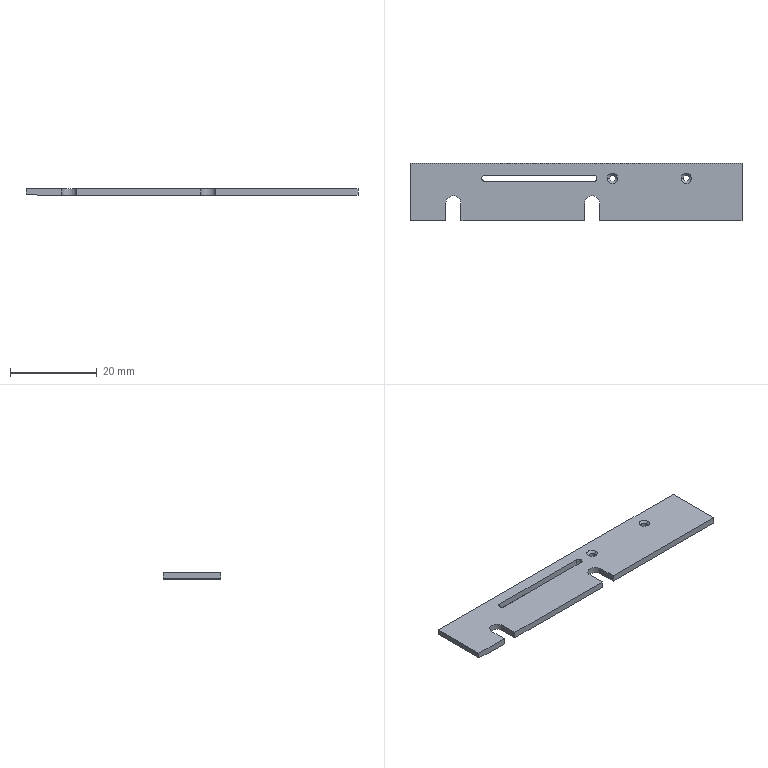Part | NX | 1 solid | 28 faces | box 76.5 x 13.2 x 1.5 mm | volume 1388 mm3 | plane 15 | cylinder 9 | cone 4 | commonest cylinder face diameters 1.4 x4 1.5 x3 3.5 x2
STEP:
#1=CARTESIAN_POINT('',(-191.15,-6.,0.75));
#2=VERTEX_POINT('',#1);
#3=CARTESIAN_POINT('',(-191.15,-2.,0.75));
#4=VERTEX_POINT('',#3);
#5=CARTESIAN_POINT('',(-191.15,0.,0.75));
#6=DIRECTION('',(0.,1.,0.));
#7=VECTOR('',#6,1000.);
#8=LINE('',#5,#7);
#9=EDGE_CURVE('',#2,#4,#8,.T.);
#10=ORIENTED_EDGE('',*,*,#9,.F.);
#11=CARTESIAN_POINT('',(-158.4,-6.,0.75));
#12=VERTEX_POINT('',#11);
#13=CARTESIAN_POINT('',(0.,-6.,0.75));
#14=DIRECTION('',(-1.,0.,0.));
#15=VECTOR('',#14,1000.);
#16=LINE('',#13,#15);
#17=EDGE_CURVE('',#12,#2,#16,.T.);
#18=ORIENTED_EDGE('',*,*,#17,.F.);
#19=CARTESIAN_POINT('',(-158.4,7.2,0.75));
#20=VERTEX_POINT('',#19);
#21=CARTESIAN_POINT('',(-158.4,0.,0.75));
#22=DIRECTION('',(0.,-1.,0.));
#23=VECTOR('',#22,1000.);
#24=LINE('',#21,#23);
#25=EDGE_CURVE('',#20,#12,#24,.T.);
#26=ORIENTED_EDGE('',*,*,#25,.F.);
#27=CARTESIAN_POINT('',(-234.9,7.2,0.75));
#28=VERTEX_POINT('',#27);
#29=CARTESIAN_POINT('',(0.,7.2,0.75));
#30=DIRECTION('',(1.,0.,0.));
#31=VECTOR('',#30,1000.);
#32=LINE('',#29,#31);
#33=EDGE_CURVE('',#28,#20,#32,.T.);
#34=ORIENTED_EDGE('',*,*,#33,.F.);
#35=CARTESIAN_POINT('',(-234.9,-6.,0.75));
#36=VERTEX_POINT('',#35);
#37=CARTESIAN_POINT('',(-234.9,0.,0.75));
#38=DIRECTION('',(0.,1.,0.));
#39=VECTOR('',#38,1000.);
#40=LINE('',#37,#39);
#41=EDGE_CURVE('',#36,#28,#40,.T.);
#42=ORIENTED_EDGE('',*,*,#41,.F.);
#43=CARTESIAN_POINT('',(-226.65,-6.,0.75));
#44=VERTEX_POINT('',#43);
#45=CARTESIAN_POINT('',(0.,-6.,0.75));
#46=DIRECTION('',(-1.,0.,0.));
#47=VECTOR('',#46,1000.);
#48=LINE('',#45,#47);
#49=EDGE_CURVE('',#44,#36,#48,.T.);
#50=ORIENTED_EDGE('',*,*,#49,.F.);
#51=CARTESIAN_POINT('',(-226.65,-2.,0.75));
#52=VERTEX_POINT('',#51);
#53=CARTESIAN_POINT('',(-226.65,0.,0.75));
#54=DIRECTION('',(0.,-1.,0.));
#55=VECTOR('',#54,1000.);
#56=LINE('',#53,#55);
#57=EDGE_CURVE('',#52,#44,#56,.T.);
#58=ORIENTED_EDGE('',*,*,#57,.F.);
#59=CARTESIAN_POINT('',(-223.15,-2.,0.75));
#60=VERTEX_POINT('',#59);
#61=CARTESIAN_POINT('',(-224.9,-2.,0.75));
#62=DIRECTION('',(0.,0.,-1.));
#63=DIRECTION('',(-1.,0.,0.));
#64=AXIS2_PLACEMENT_3D('',#61,#62,#63);
#65=CIRCLE('',#64,1.75);
#66=EDGE_CURVE('',#52,#60,#65,.T.);
#67=ORIENTED_EDGE('',*,*,#66,.T.);
#68=CARTESIAN_POINT('',(-223.15,-6.,0.75));
#69=VERTEX_POINT('',#68);
#70=CARTESIAN_POINT('',(-223.15,0.,0.75));
#71=DIRECTION('',(0.,1.,0.));
#72=VECTOR('',#71,1000.);
#73=LINE('',#70,#72);
#74=EDGE_CURVE('',#69,#60,#73,.T.);
#75=ORIENTED_EDGE('',*,*,#74,.F.);
#76=CARTESIAN_POINT('',(-194.65,-6.,0.75));
#77=VERTEX_POINT('',#76);
#78=CARTESIAN_POINT('',(0.,-6.,0.75));
#79=DIRECTION('',(-1.,0.,0.));
#80=VECTOR('',#79,1000.);
#81=LINE('',#78,#80);
#82=EDGE_CURVE('',#77,#69,#81,.T.);
#83=ORIENTED_EDGE('',*,*,#82,.F.);
#84=CARTESIAN_POINT('',(-194.65,-2.,0.75));
#85=VERTEX_POINT('',#84);
#86=CARTESIAN_POINT('',(-194.65,0.,0.75));
#87=DIRECTION('',(0.,-1.,0.));
#88=VECTOR('',#87,1000.);
#89=LINE('',#86,#88);
#90=EDGE_CURVE('',#85,#77,#89,.T.);
#91=ORIENTED_EDGE('',*,*,#90,.F.);
#92=CARTESIAN_POINT('',(-192.9,-2.,0.75));
#93=DIRECTION('',(0.,0.,-1.));
#94=DIRECTION('',(-1.,0.,0.));
#95=AXIS2_PLACEMENT_3D('',#92,#93,#94);
#96=CIRCLE('',#95,1.75);
#97=EDGE_CURVE('',#85,#4,#96,.T.);
#98=ORIENTED_EDGE('',*,*,#97,.T.);
#99=EDGE_LOOP('',(#10,#18,#26,#34,#42,#50,#58,#67,#75,#83,#91,#98));
#100=FACE_BOUND('',#99,.T.);
#101=CARTESIAN_POINT('',(-192.6,3.,0.75));
#102=VERTEX_POINT('',#101);
#103=CARTESIAN_POINT('',(-192.6,4.5,0.75));
#104=VERTEX_POINT('',#103);
#105=CARTESIAN_POINT('',(-192.6,3.75,0.75));
#106=DIRECTION('',(0.,0.,1.));
#107=DIRECTION('',(-1.,0.,0.));
#108=AXIS2_PLACEMENT_3D('',#105,#106,#107);
#109=CIRCLE('',#108,0.75);
#110=EDGE_CURVE('',#102,#104,#109,.T.);
#111=ORIENTED_EDGE('',*,*,#110,.F.);
#112=CARTESIAN_POINT('',(-217.6,3.,0.75));
#113=VERTEX_POINT('',#112);
#114=CARTESIAN_POINT('',(0.,3.,0.75));
#115=DIRECTION('',(1.,0.,0.));
#116=VECTOR('',#115,1000.);
#117=LINE('',#114,#116);
#118=EDGE_CURVE('',#113,#102,#117,.T.);
#119=ORIENTED_EDGE('',*,*,#118,.F.);
#120=CARTESIAN_POINT('',(-218.35,3.75,0.75));
#121=VERTEX_POINT('',#120);
#122=CARTESIAN_POINT('',(-217.6,3.75,0.75));
#123=DIRECTION('',(0.,0.,1.));
#124=DIRECTION('',(-1.,0.,0.));
#125=AXIS2_PLACEMENT_3D('',#122,#123,#124);
#126=CIRCLE('',#125,0.75);
#127=EDGE_CURVE('',#121,#113,#126,.T.);
#128=ORIENTED_EDGE('',*,*,#127,.F.);
#129=CARTESIAN_POINT('',(-217.6,4.5,0.75));
#130=VERTEX_POINT('',#129);
#131=CARTESIAN_POINT('',(-217.6,3.75,0.75));
#132=DIRECTION('',(0.,0.,1.));
#133=DIRECTION('',(-1.,0.,0.));
#134=AXIS2_PLACEMENT_3D('',#131,#132,#133);
#135=CIRCLE('',#134,0.75);
#136=EDGE_CURVE('',#130,#121,#135,.T.);
#137=ORIENTED_EDGE('',*,*,#136,.F.);
#138=CARTESIAN_POINT('',(0.,4.5,0.75));
#139=DIRECTION('',(-1.,0.,0.));
#140=VECTOR('',#139,1000.);
#141=LINE('',#138,#140);
#142=EDGE_CURVE('',#104,#130,#141,.T.);
#143=ORIENTED_EDGE('',*,*,#142,.F.);
#144=EDGE_LOOP('',(#111,#119,#128,#137,#143));
#145=FACE_BOUND('',#144,.T.);
#146=CARTESIAN_POINT('',(-189.45,3.75,0.75));
#147=VERTEX_POINT('',#146);
#148=CARTESIAN_POINT('',(-187.05,3.75,0.75));
#149=VERTEX_POINT('',#148);
#150=CARTESIAN_POINT('',(-188.25,3.75,0.75));
#151=DIRECTION('',(0.,0.,1.));
#152=DIRECTION('',(1.,0.,0.));
#153=AXIS2_PLACEMENT_3D('',#150,#151,#152);
#154=CIRCLE('',#153,1.2);
#155=EDGE_CURVE('',#147,#149,#154,.T.);
#156=ORIENTED_EDGE('',*,*,#155,.F.);
#157=CARTESIAN_POINT('',(-188.25,3.75,0.75));
#158=DIRECTION('',(0.,0.,1.));
#159=DIRECTION('',(1.,0.,0.));
#160=AXIS2_PLACEMENT_3D('',#157,#158,#159);
#161=CIRCLE('',#160,1.2);
#162=EDGE_CURVE('',#149,#147,#161,.T.);
#163=ORIENTED_EDGE('',*,*,#162,.F.);
#164=EDGE_LOOP('',(#156,#163));
#165=FACE_BOUND('',#164,.T.);
#166=CARTESIAN_POINT('',(-172.45,3.75,0.75));
#167=VERTEX_POINT('',#166);
#168=CARTESIAN_POINT('',(-170.05,3.75,0.75));
#169=VERTEX_POINT('',#168);
#170=CARTESIAN_POINT('',(-171.25,3.75,0.75));
#171=DIRECTION('',(0.,0.,1.));
#172=DIRECTION('',(1.,0.,0.));
#173=AXIS2_PLACEMENT_3D('',#170,#171,#172);
#174=CIRCLE('',#173,1.2);
#175=EDGE_CURVE('',#167,#169,#174,.T.);
#176=ORIENTED_EDGE('',*,*,#175,.F.);
#177=CARTESIAN_POINT('',(-171.25,3.75,0.75));
#178=DIRECTION('',(0.,0.,1.));
#179=DIRECTION('',(1.,0.,0.));
#180=AXIS2_PLACEMENT_3D('',#177,#178,#179);
#181=CIRCLE('',#180,1.2);
#182=EDGE_CURVE('',#169,#167,#181,.T.);
#183=ORIENTED_EDGE('',*,*,#182,.F.);
#184=EDGE_LOOP('',(#176,#183));
#185=FACE_BOUND('',#184,.T.);
#186=CARTESIAN_POINT('',(-196.6,0.,0.75));
#187=DIRECTION('',(0.,0.,-1.));
#188=DIRECTION('',(0.,-1.,0.));
#189=AXIS2_PLACEMENT_3D('',#186,#187,#188);
#190=PLANE('',#189);
#191=ADVANCED_FACE('',(#100,#145,#165,#185),#190,.F.);
#192=CARTESIAN_POINT('',(-191.15,-6.,-0.75));
#193=VERTEX_POINT('',#192);
#194=CARTESIAN_POINT('',(-191.15,-2.,-0.75));
#195=VERTEX_POINT('',#194);
#196=CARTESIAN_POINT('',(-191.15,0.,-0.75));
#197=DIRECTION('',(0.,1.,0.));
#198=VECTOR('',#197,1000.);
#199=LINE('',#196,#198);
#200=EDGE_CURVE('',#193,#195,#199,.T.);
#201=ORIENTED_EDGE('',*,*,#200,.F.);
#202=CARTESIAN_POINT('',(-191.15,-6.,0.));
#203=DIRECTION('',(0.,0.,1.));
#204=VECTOR('',#203,1000.);
#205=LINE('',#202,#204);
#206=EDGE_CURVE('',#193,#2,#205,.T.);
#207=ORIENTED_EDGE('',*,*,#206,.T.);
#208=ORIENTED_EDGE('',*,*,#9,.T.);
#209=CARTESIAN_POINT('',(-191.15,-2.,0.75));
#210=DIRECTION('',(0.,0.,-1.));
#211=VECTOR('',#210,1000.);
#212=LINE('',#209,#211);
#213=EDGE_CURVE('',#4,#195,#212,.T.);
#214=ORIENTED_EDGE('',*,*,#213,.T.);
#215=EDGE_LOOP('',(#201,#207,#208,#214));
#216=FACE_BOUND('',#215,.T.);
#217=CARTESIAN_POINT('',(-191.15,-6.,0.75));
#218=DIRECTION('',(1.,0.,0.));
#219=DIRECTION('',(0.,1.,0.));
#220=AXIS2_PLACEMENT_3D('',#217,#218,#219);
#221=PLANE('',#220);
#222=ADVANCED_FACE('',(#216),#221,.F.);
#223=ORIENTED_EDGE('',*,*,#213,.F.);
#224=ORIENTED_EDGE('',*,*,#97,.F.);
#225=CARTESIAN_POINT('',(-194.65,-2.,-0.75));
#226=VERTEX_POINT('',#225);
#227=CARTESIAN_POINT('',(-194.65,-2.,0.75));
#228=DIRECTION('',(0.,0.,-1.));
#229=VECTOR('',#228,1000.);
#230=LINE('',#227,#229);
#231=EDGE_CURVE('',#85,#226,#230,.T.);
#232=ORIENTED_EDGE('',*,*,#231,.T.);
#233=CARTESIAN_POINT('',(-192.9,-2.,-0.75));
#234=DIRECTION('',(0.,0.,-1.));
#235=DIRECTION('',(-1.,0.,0.));
#236=AXIS2_PLACEMENT_3D('',#233,#234,#235);
#237=CIRCLE('',#236,1.75);
#238=EDGE_CURVE('',#226,#195,#237,.T.);
#239=ORIENTED_EDGE('',*,*,#238,.T.);
#240=EDGE_LOOP('',(#223,#224,#232,#239));
#241=FACE_BOUND('',#240,.T.);
#242=CARTESIAN_POINT('',(-192.9,-2.,0.75));
#243=DIRECTION('',(0.,0.,-1.));
#244=DIRECTION('',(-1.,0.,0.));
#245=AXIS2_PLACEMENT_3D('',#242,#243,#244);
#246=CYLINDRICAL_SURFACE('',#245,1.75);
#247=ADVANCED_FACE('',(#241),#246,.F.);
#248=CARTESIAN_POINT('',(-194.65,-6.,-0.75));
#249=VERTEX_POINT('',#248);
#250=CARTESIAN_POINT('',(-194.65,0.,-0.75));
#251=DIRECTION('',(0.,-1.,0.));
#252=VECTOR('',#251,1000.);
#253=LINE('',#250,#252);
#254=EDGE_CURVE('',#226,#249,#253,.T.);
#255=ORIENTED_EDGE('',*,*,#254,.F.);
#256=ORIENTED_EDGE('',*,*,#231,.F.);
#257=ORIENTED_EDGE('',*,*,#90,.T.);
#258=CARTESIAN_POINT('',(-194.65,-6.,0.75));
#259=DIRECTION('',(0.,0.,-1.));
#260=VECTOR('',#259,1000.);
#261=LINE('',#258,#260);
#262=EDGE_CURVE('',#77,#249,#261,.T.);
#263=ORIENTED_EDGE('',*,*,#262,.T.);
#264=EDGE_LOOP('',(#255,#256,#257,#263));
#265=FACE_BOUND('',#264,.T.);
#266=CARTESIAN_POINT('',(-194.65,-2.,0.75));
#267=DIRECTION('',(-1.,0.,0.));
#268=DIRECTION('',(0.,0.,1.));
#269=AXIS2_PLACEMENT_3D('',#266,#267,#268);
#270=PLANE('',#269);
#271=ADVANCED_FACE('',(#265),#270,.F.);
#272=ORIENTED_EDGE('',*,*,#262,.F.);
#273=ORIENTED_EDGE('',*,*,#82,.T.);
#274=CARTESIAN_POINT('',(-223.15,-6.,-0.75));
#275=VERTEX_POINT('',#274);
#276=CARTESIAN_POINT('',(-223.15,-6.,0.75));
#277=DIRECTION('',(0.,0.,-1.));
#278=VECTOR('',#277,1000.);
#279=LINE('',#276,#278);
#280=EDGE_CURVE('',#69,#275,#279,.T.);
#281=ORIENTED_EDGE('',*,*,#280,.T.);
#282=CARTESIAN_POINT('',(0.,-6.,-0.75));
#283=DIRECTION('',(-1.,0.,0.));
#284=VECTOR('',#283,1000.);
#285=LINE('',#282,#284);
#286=EDGE_CURVE('',#249,#275,#285,.T.);
#287=ORIENTED_EDGE('',*,*,#286,.F.);
#288=EDGE_LOOP('',(#272,#273,#281,#287));
#289=FACE_BOUND('',#288,.T.);
#290=CARTESIAN_POINT('',(-158.3,-6.,-0.75));
#291=DIRECTION('',(0.,1.,0.));
#292=DIRECTION('',(1.,0.,0.));
#293=AXIS2_PLACEMENT_3D('',#290,#291,#292);
#294=PLANE('',#293);
#295=ADVANCED_FACE('',(#289),#294,.F.);
#296=CARTESIAN_POINT('',(-223.15,-2.,-0.75));
#297=VERTEX_POINT('',#296);
#298=CARTESIAN_POINT('',(-223.15,0.,-0.75));
#299=DIRECTION('',(0.,1.,0.));
#300=VECTOR('',#299,1000.);
#301=LINE('',#298,#300);
#302=EDGE_CURVE('',#275,#297,#301,.T.);
#303=ORIENTED_EDGE('',*,*,#302,.F.);
#304=ORIENTED_EDGE('',*,*,#280,.F.);
#305=ORIENTED_EDGE('',*,*,#74,.T.);
#306=CARTESIAN_POINT('',(-223.15,-2.,0.75));
#307=DIRECTION('',(0.,0.,-1.));
#308=VECTOR('',#307,1000.);
#309=LINE('',#306,#308);
#310=EDGE_CURVE('',#60,#297,#309,.T.);
#311=ORIENTED_EDGE('',*,*,#310,.T.);
#312=EDGE_LOOP('',(#303,#304,#305,#311));
#313=FACE_BOUND('',#312,.T.);
#314=CARTESIAN_POINT('',(-223.15,-6.,0.75));
#315=DIRECTION('',(1.,0.,0.));
#316=DIRECTION('',(0.,1.,0.));
#317=AXIS2_PLACEMENT_3D('',#314,#315,#316);
#318=PLANE('',#317);
#319=ADVANCED_FACE('',(#313),#318,.F.);
#320=ORIENTED_EDGE('',*,*,#310,.F.);
#321=ORIENTED_EDGE('',*,*,#66,.F.);
#322=CARTESIAN_POINT('',(-226.65,-2.,-0.75));
#323=VERTEX_POINT('',#322);
#324=CARTESIAN_POINT('',(-226.65,-2.,0.75));
#325=DIRECTION('',(0.,0.,-1.));
#326=VECTOR('',#325,1000.);
#327=LINE('',#324,#326);
#328=EDGE_CURVE('',#52,#323,#327,.T.);
#329=ORIENTED_EDGE('',*,*,#328,.T.);
#330=CARTESIAN_POINT('',(-224.9,-2.,-0.75));
#331=DIRECTION('',(0.,0.,-1.));
#332=DIRECTION('',(-1.,0.,0.));
#333=AXIS2_PLACEMENT_3D('',#330,#331,#332);
#334=CIRCLE('',#333,1.75);
#335=EDGE_CURVE('',#323,#297,#334,.T.);
#336=ORIENTED_EDGE('',*,*,#335,.T.);
#337=EDGE_LOOP('',(#320,#321,#329,#336));
#338=FACE_BOUND('',#337,.T.);
#339=CARTESIAN_POINT('',(-224.9,-2.,0.75));
#340=DIRECTION('',(0.,0.,-1.));
#341=DIRECTION('',(-1.,0.,0.));
#342=AXIS2_PLACEMENT_3D('',#339,#340,#341);
#343=CYLINDRICAL_SURFACE('',#342,1.75);
#344=ADVANCED_FACE('',(#338),#343,.F.);
#345=CARTESIAN_POINT('',(-226.65,-6.,-0.75));
#346=VERTEX_POINT('',#345);
#347=CARTESIAN_POINT('',(-226.65,0.,-0.75));
#348=DIRECTION('',(0.,-1.,0.));
#349=VECTOR('',#348,1000.);
#350=LINE('',#347,#349);
#351=EDGE_CURVE('',#323,#346,#350,.T.);
#352=ORIENTED_EDGE('',*,*,#351,.F.);
#353=ORIENTED_EDGE('',*,*,#328,.F.);
#354=ORIENTED_EDGE('',*,*,#57,.T.);
#355=CARTESIAN_POINT('',(-226.65,-6.,0.75));
#356=DIRECTION('',(0.,0.,-1.));
#357=VECTOR('',#356,1000.);
#358=LINE('',#355,#357);
#359=EDGE_CURVE('',#44,#346,#358,.T.);
#360=ORIENTED_EDGE('',*,*,#359,.T.);
#361=EDGE_LOOP('',(#352,#353,#354,#360));
#362=FACE_BOUND('',#361,.T.);
#363=CARTESIAN_POINT('',(-226.65,-2.,0.75));
#364=DIRECTION('',(-1.,0.,0.));
#365=DIRECTION('',(0.,0.,1.));
#366=AXIS2_PLACEMENT_3D('',#363,#364,#365);
#367=PLANE('',#366);
#368=ADVANCED_FACE('',(#362),#367,.F.);
#369=ORIENTED_EDGE('',*,*,#359,.F.);
#370=ORIENTED_EDGE('',*,*,#49,.T.);
#371=CARTESIAN_POINT('',(-234.9,-6.,-0.4875));
#372=VERTEX_POINT('',#371);
#373=CARTESIAN_POINT('',(-234.9,-6.,0.));
#374=DIRECTION('',(0.,0.,-1.));
#375=VECTOR('',#374,1000.);
#376=LINE('',#373,#375);
#377=EDGE_CURVE('',#36,#372,#376,.T.);
#378=ORIENTED_EDGE('',*,*,#377,.T.);
#379=CARTESIAN_POINT('',(-231.9,-6.,-0.75));
#380=VERTEX_POINT('',#379);
#381=CARTESIAN_POINT('',(0.,-6.,-21.039));
#382=DIRECTION('',(0.9962,0.,-0.08716));
#383=VECTOR('',#382,1000.);
#384=LINE('',#381,#383);
#385=EDGE_CURVE('',#372,#380,#384,.T.);
#386=ORIENTED_EDGE('',*,*,#385,.T.);
#387=CARTESIAN_POINT('',(0.,-6.,-0.75));
#388=DIRECTION('',(-1.,0.,0.));
#389=VECTOR('',#388,1000.);
#390=LINE('',#387,#389);
#391=EDGE_CURVE('',#346,#380,#390,.T.);
#392=ORIENTED_EDGE('',*,*,#391,.F.);
#393=EDGE_LOOP('',(#369,#370,#378,#386,#392));
#394=FACE_BOUND('',#393,.T.);
#395=CARTESIAN_POINT('',(-158.3,-6.,-0.75));
#396=DIRECTION('',(0.,1.,0.));
#397=DIRECTION('',(1.,0.,0.));
#398=AXIS2_PLACEMENT_3D('',#395,#396,#397);
#399=PLANE('',#398);
#400=ADVANCED_FACE('',(#394),#399,.F.);
#401=CARTESIAN_POINT('',(-231.9,7.2,-0.75));
#402=VERTEX_POINT('',#401);
#403=CARTESIAN_POINT('',(-231.9,0.,-0.75));
#404=DIRECTION('',(0.,1.,0.));
#405=VECTOR('',#404,1000.);
#406=LINE('',#403,#405);
#407=EDGE_CURVE('',#380,#402,#406,.T.);
#408=ORIENTED_EDGE('',*,*,#407,.F.);
#409=ORIENTED_EDGE('',*,*,#385,.F.);
#410=CARTESIAN_POINT('',(-234.9,7.2,-0.4875));
#411=VERTEX_POINT('',#410);
#412=CARTESIAN_POINT('',(-234.9,0.,-0.4875));
#413=DIRECTION('',(0.,1.,0.));
#414=VECTOR('',#413,1000.);
#415=LINE('',#412,#414);
#416=EDGE_CURVE('',#372,#411,#415,.T.);
#417=ORIENTED_EDGE('',*,*,#416,.T.);
#418=CARTESIAN_POINT('',(0.,7.2,-21.039));
#419=DIRECTION('',(0.9962,0.,-0.08716));
#420=VECTOR('',#419,1000.);
#421=LINE('',#418,#420);
#422=EDGE_CURVE('',#411,#402,#421,.T.);
#423=ORIENTED_EDGE('',*,*,#422,.T.);
#424=EDGE_LOOP('',(#408,#409,#417,#423));
#425=FACE_BOUND('',#424,.T.);
#426=CARTESIAN_POINT('',(-231.9,-6.,-0.75));
#427=DIRECTION('',(0.08716,0.,0.9962));
#428=DIRECTION('',(0.,-1.,0.));
#429=AXIS2_PLACEMENT_3D('',#426,#427,#428);
#430=PLANE('',#429);
#431=ADVANCED_FACE('',(#425),#430,.F.);
#432=CARTESIAN_POINT('',(-158.4,7.2,-0.75));
#433=VERTEX_POINT('',#432);
#434=CARTESIAN_POINT('',(0.,7.2,-0.75));
#435=DIRECTION('',(1.,0.,0.));
#436=VECTOR('',#435,1000.);
#437=LINE('',#434,#436);
#438=EDGE_CURVE('',#402,#433,#437,.T.);
#439=ORIENTED_EDGE('',*,*,#438,.F.);
#440=ORIENTED_EDGE('',*,*,#422,.F.);
#441=CARTESIAN_POINT('',(-234.9,7.2,0.));
#442=DIRECTION('',(0.,0.,-1.));
#443=VECTOR('',#442,1000.);
#444=LINE('',#441,#443);
#445=EDGE_CURVE('',#28,#411,#444,.T.);
#446=ORIENTED_EDGE('',*,*,#445,.F.);
#447=ORIENTED_EDGE('',*,*,#33,.T.);
#448=CARTESIAN_POINT('',(-158.4,7.2,0.));
#449=DIRECTION('',(0.,0.,-1.));
#450=VECTOR('',#449,1000.);
#451=LINE('',#448,#450);
#452=EDGE_CURVE('',#20,#433,#451,.T.);
#453=ORIENTED_EDGE('',*,*,#452,.T.);
#454=EDGE_LOOP('',(#439,#440,#446,#447,#453));
#455=FACE_BOUND('',#454,.T.);
#456=CARTESIAN_POINT('',(-234.9,7.2,-0.75));
#457=DIRECTION('',(0.,-1.,0.));
#458=DIRECTION('',(0.,0.,-1.));
#459=AXIS2_PLACEMENT_3D('',#456,#457,#458);
#460=PLANE('',#459);
#461=ADVANCED_FACE('',(#455),#460,.F.);
#462=CARTESIAN_POINT('',(-158.4,-6.,-0.75));
#463=VERTEX_POINT('',#462);
#464=CARTESIAN_POINT('',(-158.4,0.,-0.75));
#465=DIRECTION('',(0.,-1.,0.));
#466=VECTOR('',#465,1000.);
#467=LINE('',#464,#466);
#468=EDGE_CURVE('',#433,#463,#467,.T.);
#469=ORIENTED_EDGE('',*,*,#468,.F.);
#470=ORIENTED_EDGE('',*,*,#452,.F.);
#471=ORIENTED_EDGE('',*,*,#25,.T.);
#472=CARTESIAN_POINT('',(-158.4,-6.,0.));
#473=DIRECTION('',(0.,0.,1.));
#474=VECTOR('',#473,1000.);
#475=LINE('',#472,#474);
#476=EDGE_CURVE('',#463,#12,#475,.T.);
#477=ORIENTED_EDGE('',*,*,#476,.F.);
#478=EDGE_LOOP('',(#469,#470,#471,#477));
#479=FACE_BOUND('',#478,.T.);
#480=CARTESIAN_POINT('',(-158.4,6.,-0.75));
#481=DIRECTION('',(-1.,0.,0.));
#482=DIRECTION('',(0.,0.,1.));
#483=AXIS2_PLACEMENT_3D('',#480,#481,#482);
#484=PLANE('',#483);
#485=ADVANCED_FACE('',(#479),#484,.F.);
#486=ORIENTED_EDGE('',*,*,#206,.F.);
#487=CARTESIAN_POINT('',(0.,-6.,-0.75));
#488=DIRECTION('',(-1.,0.,0.));
#489=VECTOR('',#488,1000.);
#490=LINE('',#487,#489);
#491=EDGE_CURVE('',#463,#193,#490,.T.);
#492=ORIENTED_EDGE('',*,*,#491,.F.);
#493=ORIENTED_EDGE('',*,*,#476,.T.);
#494=ORIENTED_EDGE('',*,*,#17,.T.);
#495=EDGE_LOOP('',(#486,#492,#493,#494));
#496=FACE_BOUND('',#495,.T.);
#497=CARTESIAN_POINT('',(-158.3,-6.,-0.75));
#498=DIRECTION('',(0.,1.,0.));
#499=DIRECTION('',(1.,0.,0.));
#500=AXIS2_PLACEMENT_3D('',#497,#498,#499);
#501=PLANE('',#500);
#502=ADVANCED_FACE('',(#496),#501,.F.);
#503=ORIENTED_EDGE('',*,*,#200,.T.);
#504=ORIENTED_EDGE('',*,*,#238,.F.);
#505=ORIENTED_EDGE('',*,*,#254,.T.);
#506=ORIENTED_EDGE('',*,*,#286,.T.);
#507=ORIENTED_EDGE('',*,*,#302,.T.);
#508=ORIENTED_EDGE('',*,*,#335,.F.);
#509=ORIENTED_EDGE('',*,*,#351,.T.);
#510=ORIENTED_EDGE('',*,*,#391,.T.);
#511=ORIENTED_EDGE('',*,*,#407,.T.);
#512=ORIENTED_EDGE('',*,*,#438,.T.);
#513=ORIENTED_EDGE('',*,*,#468,.T.);
#514=ORIENTED_EDGE('',*,*,#491,.T.);
#515=EDGE_LOOP('',(#503,#504,#505,#506,#507,#508,#509,#510,#511,#512,#513,#514));
#516=FACE_BOUND('',#515,.T.);
#517=CARTESIAN_POINT('',(-187.55,3.75,-0.75));
#518=VERTEX_POINT('',#517);
#519=CARTESIAN_POINT('',(-188.95,3.75,-0.75));
#520=VERTEX_POINT('',#519);
#521=CARTESIAN_POINT('',(-188.25,3.75,-0.75));
#522=DIRECTION('',(0.,0.,-1.));
#523=DIRECTION('',(-1.,0.,0.));
#524=AXIS2_PLACEMENT_3D('',#521,#522,#523);
#525=CIRCLE('',#524,0.7);
#526=EDGE_CURVE('',#518,#520,#525,.T.);
#527=ORIENTED_EDGE('',*,*,#526,.F.);
#528=CARTESIAN_POINT('',(-188.25,3.75,-0.75));
#529=DIRECTION('',(0.,0.,-1.));
#530=DIRECTION('',(-1.,0.,0.));
#531=AXIS2_PLACEMENT_3D('',#528,#529,#530);
#532=CIRCLE('',#531,0.7);
#533=EDGE_CURVE('',#520,#518,#532,.T.);
#534=ORIENTED_EDGE('',*,*,#533,.F.);
#535=EDGE_LOOP('',(#527,#534));
#536=FACE_BOUND('',#535,.T.);
#537=CARTESIAN_POINT('',(-192.6,3.,-0.75));
#538=VERTEX_POINT('',#537);
#539=CARTESIAN_POINT('',(-192.6,4.5,-0.75));
#540=VERTEX_POINT('',#539);
#541=CARTESIAN_POINT('',(-192.6,3.75,-0.75));
#542=DIRECTION('',(0.,0.,1.));
#543=DIRECTION('',(-1.,0.,0.));
#544=AXIS2_PLACEMENT_3D('',#541,#542,#543);
#545=CIRCLE('',#544,0.75);
#546=EDGE_CURVE('',#538,#540,#545,.T.);
#547=ORIENTED_EDGE('',*,*,#546,.T.);
#548=CARTESIAN_POINT('',(-217.6,4.5,-0.75));
#549=VERTEX_POINT('',#548);
#550=CARTESIAN_POINT('',(0.,4.5,-0.75));
#551=DIRECTION('',(-1.,0.,0.));
#552=VECTOR('',#551,1000.);
#553=LINE('',#550,#552);
#554=EDGE_CURVE('',#540,#549,#553,.T.);
#555=ORIENTED_EDGE('',*,*,#554,.T.);
#556=CARTESIAN_POINT('',(-218.35,3.75,-0.75));
#557=VERTEX_POINT('',#556);
#558=CARTESIAN_POINT('',(-217.6,3.75,-0.75));
#559=DIRECTION('',(0.,0.,1.));
#560=DIRECTION('',(-1.,0.,0.));
#561=AXIS2_PLACEMENT_3D('',#558,#559,#560);
#562=CIRCLE('',#561,0.75);
#563=EDGE_CURVE('',#549,#557,#562,.T.);
#564=ORIENTED_EDGE('',*,*,#563,.T.);
#565=CARTESIAN_POINT('',(-217.6,3.,-0.75));
#566=VERTEX_POINT('',#565);
#567=CARTESIAN_POINT('',(-217.6,3.75,-0.75));
#568=DIRECTION('',(0.,0.,1.));
#569=DIRECTION('',(-1.,0.,0.));
#570=AXIS2_PLACEMENT_3D('',#567,#568,#569);
#571=CIRCLE('',#570,0.75);
#572=EDGE_CURVE('',#557,#566,#571,.T.);
#573=ORIENTED_EDGE('',*,*,#572,.T.);
#574=CARTESIAN_POINT('',(0.,3.,-0.75));
#575=DIRECTION('',(1.,0.,0.));
#576=VECTOR('',#575,1000.);
#577=LINE('',#574,#576);
#578=EDGE_CURVE('',#566,#538,#577,.T.);
#579=ORIENTED_EDGE('',*,*,#578,.T.);
#580=EDGE_LOOP('',(#547,#555,#564,#573,#579));
#581=FACE_BOUND('',#580,.T.);
#582=CARTESIAN_POINT('',(-171.95,3.75,-0.75));
#583=VERTEX_POINT('',#582);
#584=CARTESIAN_POINT('',(-170.55,3.75,-0.75));
#585=VERTEX_POINT('',#584);
#586=CARTESIAN_POINT('',(-171.25,3.75,-0.75));
#587=DIRECTION('',(0.,0.,-1.));
#588=DIRECTION('',(-1.,0.,0.));
#589=AXIS2_PLACEMENT_3D('',#586,#587,#588);
#590=CIRCLE('',#589,0.7);
#591=EDGE_CURVE('',#583,#585,#590,.T.);
#592=ORIENTED_EDGE('',*,*,#591,.F.);
#593=CARTESIAN_POINT('',(-171.25,3.75,-0.75));
#594=DIRECTION('',(0.,0.,-1.));
#595=DIRECTION('',(-1.,0.,0.));
#596=AXIS2_PLACEMENT_3D('',#593,#594,#595);
#597=CIRCLE('',#596,0.7);
#598=EDGE_CURVE('',#585,#583,#597,.T.);
#599=ORIENTED_EDGE('',*,*,#598,.F.);
#600=EDGE_LOOP('',(#592,#599));
#601=FACE_BOUND('',#600,.T.);
#602=CARTESIAN_POINT('',(-196.6,0.,-0.75));
#603=DIRECTION('',(0.,0.,-1.));
#604=DIRECTION('',(0.,-1.,0.));
#605=AXIS2_PLACEMENT_3D('',#602,#603,#604);
#606=PLANE('',#605);
#607=ADVANCED_FACE('',(#516,#536,#581,#601),#606,.T.);
#608=ORIENTED_EDGE('',*,*,#416,.F.);
#609=ORIENTED_EDGE('',*,*,#377,.F.);
#610=ORIENTED_EDGE('',*,*,#41,.T.);
#611=ORIENTED_EDGE('',*,*,#445,.T.);
#612=EDGE_LOOP('',(#608,#609,#610,#611));
#613=FACE_BOUND('',#612,.T.);
#614=CARTESIAN_POINT('',(-234.9,-6.,-0.75));
#615=DIRECTION('',(1.,0.,0.));
#616=DIRECTION('',(0.,1.,0.));
#617=AXIS2_PLACEMENT_3D('',#614,#615,#616);
#618=PLANE('',#617);
#619=ADVANCED_FACE('',(#613),#618,.F.);
#620=ORIENTED_EDGE('',*,*,#554,.F.);
#621=CARTESIAN_POINT('',(-192.6,4.5,-0.75));
#622=DIRECTION('',(0.,0.,1.));
#623=VECTOR('',#622,1000.);
#624=LINE('',#621,#623);
#625=EDGE_CURVE('',#540,#104,#624,.T.);
#626=ORIENTED_EDGE('',*,*,#625,.T.);
#627=ORIENTED_EDGE('',*,*,#142,.T.);
#628=CARTESIAN_POINT('',(-217.6,4.5,0.75));
#629=DIRECTION('',(0.,0.,-1.));
#630=VECTOR('',#629,1000.);
#631=LINE('',#628,#630);
#632=EDGE_CURVE('',#130,#549,#631,.T.);
#633=ORIENTED_EDGE('',*,*,#632,.T.);
#634=EDGE_LOOP('',(#620,#626,#627,#633));
#635=FACE_BOUND('',#634,.T.);
#636=CARTESIAN_POINT('',(-188.6,4.5,0.75));
#637=DIRECTION('',(0.,1.,0.));
#638=DIRECTION('',(1.,0.,0.));
#639=AXIS2_PLACEMENT_3D('',#636,#637,#638);
#640=PLANE('',#639);
#641=ADVANCED_FACE('',(#635),#640,.F.);
#642=CARTESIAN_POINT('',(-218.35,3.75,0.75));
#643=DIRECTION('',(0.,0.,1.));
#644=VECTOR('',#643,1000.);
#645=LINE('',#642,#644);
#646=EDGE_CURVE('',#557,#121,#645,.T.);
#647=ORIENTED_EDGE('',*,*,#646,.F.);
#648=ORIENTED_EDGE('',*,*,#563,.F.);
#649=ORIENTED_EDGE('',*,*,#632,.F.);
#650=ORIENTED_EDGE('',*,*,#136,.T.);
#651=EDGE_LOOP('',(#647,#648,#649,#650));
#652=FACE_BOUND('',#651,.T.);
#653=CARTESIAN_POINT('',(-217.6,3.75,0.75));
#654=DIRECTION('',(0.,0.,1.));
#655=DIRECTION('',(-1.,0.,0.));
#656=AXIS2_PLACEMENT_3D('',#653,#654,#655);
#657=CYLINDRICAL_SURFACE('',#656,0.75);
#658=ADVANCED_FACE('',(#652),#657,.F.);
#659=ORIENTED_EDGE('',*,*,#526,.T.);
#660=CARTESIAN_POINT('',(-188.95,3.75,0.25));
#661=VERTEX_POINT('',#660);
#662=CARTESIAN_POINT('',(-188.95,3.75,-0.75));
#663=DIRECTION('',(0.,0.,-1.));
#664=VECTOR('',#663,1000.);
#665=LINE('',#662,#664);
#666=EDGE_CURVE('',#520,#661,#665,.F.);
#667=ORIENTED_EDGE('',*,*,#666,.T.);
#668=CARTESIAN_POINT('',(-187.55,3.75,0.25));
#669=VERTEX_POINT('',#668);
#670=CARTESIAN_POINT('',(-188.25,3.75,0.25));
#671=DIRECTION('',(0.,0.,1.));
#672=DIRECTION('',(1.,0.,0.));
#673=AXIS2_PLACEMENT_3D('',#670,#671,#672);
#674=CIRCLE('',#673,0.7);
#675=EDGE_CURVE('',#661,#669,#674,.T.);
#676=ORIENTED_EDGE('',*,*,#675,.T.);
#677=CARTESIAN_POINT('',(-187.55,3.75,-0.75));
#678=DIRECTION('',(0.,0.,-1.));
#679=VECTOR('',#678,1000.);
#680=LINE('',#677,#679);
#681=EDGE_CURVE('',#518,#669,#680,.F.);
#682=ORIENTED_EDGE('',*,*,#681,.F.);
#683=EDGE_LOOP('',(#659,#667,#676,#682));
#684=FACE_BOUND('',#683,.T.);
#685=CARTESIAN_POINT('',(-188.25,3.75,-0.75));
#686=DIRECTION('',(0.,0.,-1.));
#687=DIRECTION('',(-1.,0.,0.));
#688=AXIS2_PLACEMENT_3D('',#685,#686,#687);
#689=CYLINDRICAL_SURFACE('',#688,0.7);
#690=ADVANCED_FACE('',(#684),#689,.F.);
#691=ORIENTED_EDGE('',*,*,#546,.F.);
#692=CARTESIAN_POINT('',(-192.6,3.,0.75));
#693=DIRECTION('',(0.,0.,-1.));
#694=VECTOR('',#693,1000.);
#695=LINE('',#692,#694);
#696=EDGE_CURVE('',#102,#538,#695,.T.);
#697=ORIENTED_EDGE('',*,*,#696,.F.);
#698=ORIENTED_EDGE('',*,*,#110,.T.);
#699=ORIENTED_EDGE('',*,*,#625,.F.);
#700=EDGE_LOOP('',(#691,#697,#698,#699));
#701=FACE_BOUND('',#700,.T.);
#702=CARTESIAN_POINT('',(-192.6,3.75,0.75));
#703=DIRECTION('',(0.,0.,1.));
#704=DIRECTION('',(-1.,0.,0.));
#705=AXIS2_PLACEMENT_3D('',#702,#703,#704);
#706=CYLINDRICAL_SURFACE('',#705,0.75);
#707=ADVANCED_FACE('',(#701),#706,.F.);
#708=CARTESIAN_POINT('',(-171.95,3.75,0.25));
#709=VERTEX_POINT('',#708);
#710=CARTESIAN_POINT('',(-170.55,3.75,0.25));
#711=VERTEX_POINT('',#710);
#712=CARTESIAN_POINT('',(-171.25,3.75,0.25));
#713=DIRECTION('',(0.,0.,1.));
#714=DIRECTION('',(1.,0.,0.));
#715=AXIS2_PLACEMENT_3D('',#712,#713,#714);
#716=CIRCLE('',#715,0.7);
#717=EDGE_CURVE('',#709,#711,#716,.T.);
#718=ORIENTED_EDGE('',*,*,#717,.T.);
#719=CARTESIAN_POINT('',(-170.55,3.75,-0.75));
#720=DIRECTION('',(0.,0.,-1.));
#721=VECTOR('',#720,1000.);
#722=LINE('',#719,#721);
#723=EDGE_CURVE('',#711,#585,#722,.T.);
#724=ORIENTED_EDGE('',*,*,#723,.T.);
#725=ORIENTED_EDGE('',*,*,#598,.T.);
#726=CARTESIAN_POINT('',(-171.95,3.75,-0.75));
#727=DIRECTION('',(0.,0.,-1.));
#728=VECTOR('',#727,1000.);
#729=LINE('',#726,#728);
#730=EDGE_CURVE('',#709,#583,#729,.T.);
#731=ORIENTED_EDGE('',*,*,#730,.F.);
#732=EDGE_LOOP('',(#718,#724,#725,#731));
#733=FACE_BOUND('',#732,.T.);
#734=CARTESIAN_POINT('',(-171.25,3.75,-0.75));
#735=DIRECTION('',(0.,0.,-1.));
#736=DIRECTION('',(-1.,0.,0.));
#737=AXIS2_PLACEMENT_3D('',#734,#735,#736);
#738=CYLINDRICAL_SURFACE('',#737,0.7);
#739=ADVANCED_FACE('',(#733),#738,.F.);
#740=ORIENTED_EDGE('',*,*,#578,.F.);
#741=CARTESIAN_POINT('',(-217.6,3.,-0.75));
#742=DIRECTION('',(0.,0.,1.));
#743=VECTOR('',#742,1000.);
#744=LINE('',#741,#743);
#745=EDGE_CURVE('',#566,#113,#744,.T.);
#746=ORIENTED_EDGE('',*,*,#745,.T.);
#747=ORIENTED_EDGE('',*,*,#118,.T.);
#748=ORIENTED_EDGE('',*,*,#696,.T.);
#749=EDGE_LOOP('',(#740,#746,#747,#748));
#750=FACE_BOUND('',#749,.T.);
#751=CARTESIAN_POINT('',(-211.6,3.,0.75));
#752=DIRECTION('',(0.,-1.,0.));
#753=DIRECTION('',(0.,0.,-1.));
#754=AXIS2_PLACEMENT_3D('',#751,#752,#753);
#755=PLANE('',#754);
#756=ADVANCED_FACE('',(#750),#755,.F.);
#757=ORIENTED_EDGE('',*,*,#155,.T.);
#758=CARTESIAN_POINT('',(-187.05,3.75,0.75));
#759=DIRECTION('',(0.7071,0.,0.7071));
#760=VECTOR('',#759,1000.);
#761=LINE('',#758,#760);
#762=EDGE_CURVE('',#669,#149,#761,.T.);
#763=ORIENTED_EDGE('',*,*,#762,.F.);
#764=ORIENTED_EDGE('',*,*,#675,.F.);
#765=CARTESIAN_POINT('',(-189.45,3.75,0.75));
#766=DIRECTION('',(-0.7071,0.,0.7071));
#767=VECTOR('',#766,1000.);
#768=LINE('',#765,#767);
#769=EDGE_CURVE('',#661,#147,#768,.T.);
#770=ORIENTED_EDGE('',*,*,#769,.T.);
#771=EDGE_LOOP('',(#757,#763,#764,#770));
#772=FACE_BOUND('',#771,.T.);
#773=CARTESIAN_POINT('',(-188.25,3.75,0.75));
#774=DIRECTION('',(0.,0.,1.));
#775=DIRECTION('',(1.,0.,0.));
#776=AXIS2_PLACEMENT_3D('',#773,#774,#775);
#777=CONICAL_SURFACE('',#776,1.2,0.7854);
#778=ADVANCED_FACE('',(#772),#777,.F.);
#779=ORIENTED_EDGE('',*,*,#717,.F.);
#780=CARTESIAN_POINT('',(-172.45,3.75,0.75));
#781=DIRECTION('',(-0.7071,0.,0.7071));
#782=VECTOR('',#781,1000.);
#783=LINE('',#780,#782);
#784=EDGE_CURVE('',#709,#167,#783,.T.);
#785=ORIENTED_EDGE('',*,*,#784,.T.);
#786=ORIENTED_EDGE('',*,*,#175,.T.);
#787=CARTESIAN_POINT('',(-170.05,3.75,0.75));
#788=DIRECTION('',(0.7071,0.,0.7071));
#789=VECTOR('',#788,1000.);
#790=LINE('',#787,#789);
#791=EDGE_CURVE('',#711,#169,#790,.T.);
#792=ORIENTED_EDGE('',*,*,#791,.F.);
#793=EDGE_LOOP('',(#779,#785,#786,#792));
#794=FACE_BOUND('',#793,.T.);
#795=CARTESIAN_POINT('',(-171.25,3.75,0.75));
#796=DIRECTION('',(0.,0.,1.));
#797=DIRECTION('',(1.,0.,0.));
#798=AXIS2_PLACEMENT_3D('',#795,#796,#797);
#799=CONICAL_SURFACE('',#798,1.2,0.7854);
#800=ADVANCED_FACE('',(#794),#799,.F.);
#801=ORIENTED_EDGE('',*,*,#762,.T.);
#802=ORIENTED_EDGE('',*,*,#162,.T.);
#803=ORIENTED_EDGE('',*,*,#769,.F.);
#804=CARTESIAN_POINT('',(-188.25,3.75,0.25));
#805=DIRECTION('',(0.,0.,1.));
#806=DIRECTION('',(1.,0.,0.));
#807=AXIS2_PLACEMENT_3D('',#804,#805,#806);
#808=CIRCLE('',#807,0.7);
#809=EDGE_CURVE('',#669,#661,#808,.T.);
#810=ORIENTED_EDGE('',*,*,#809,.F.);
#811=EDGE_LOOP('',(#801,#802,#803,#810));
#812=FACE_BOUND('',#811,.T.);
#813=CARTESIAN_POINT('',(-188.25,3.75,0.75));
#814=DIRECTION('',(0.,0.,1.));
#815=DIRECTION('',(1.,0.,0.));
#816=AXIS2_PLACEMENT_3D('',#813,#814,#815);
#817=CONICAL_SURFACE('',#816,1.2,0.7854);
#818=ADVANCED_FACE('',(#812),#817,.F.);
#819=ORIENTED_EDGE('',*,*,#791,.T.);
#820=ORIENTED_EDGE('',*,*,#182,.T.);
#821=ORIENTED_EDGE('',*,*,#784,.F.);
#822=CARTESIAN_POINT('',(-171.25,3.75,0.25));
#823=DIRECTION('',(0.,0.,1.));
#824=DIRECTION('',(1.,0.,0.));
#825=AXIS2_PLACEMENT_3D('',#822,#823,#824);
#826=CIRCLE('',#825,0.7);
#827=EDGE_CURVE('',#711,#709,#826,.T.);
#828=ORIENTED_EDGE('',*,*,#827,.F.);
#829=EDGE_LOOP('',(#819,#820,#821,#828));
#830=FACE_BOUND('',#829,.T.);
#831=CARTESIAN_POINT('',(-171.25,3.75,0.75));
#832=DIRECTION('',(0.,0.,1.));
#833=DIRECTION('',(1.,0.,0.));
#834=AXIS2_PLACEMENT_3D('',#831,#832,#833);
#835=CONICAL_SURFACE('',#834,1.2,0.7854);
#836=ADVANCED_FACE('',(#830),#835,.F.);
#837=ORIENTED_EDGE('',*,*,#666,.F.);
#838=ORIENTED_EDGE('',*,*,#533,.T.);
#839=ORIENTED_EDGE('',*,*,#681,.T.);
#840=ORIENTED_EDGE('',*,*,#809,.T.);
#841=EDGE_LOOP('',(#837,#838,#839,#840));
#842=FACE_BOUND('',#841,.T.);
#843=CARTESIAN_POINT('',(-188.25,3.75,-0.75));
#844=DIRECTION('',(0.,0.,-1.));
#845=DIRECTION('',(-1.,0.,0.));
#846=AXIS2_PLACEMENT_3D('',#843,#844,#845);
#847=CYLINDRICAL_SURFACE('',#846,0.7);
#848=ADVANCED_FACE('',(#842),#847,.F.);
#849=ORIENTED_EDGE('',*,*,#591,.T.);
#850=ORIENTED_EDGE('',*,*,#723,.F.);
#851=ORIENTED_EDGE('',*,*,#827,.T.);
#852=ORIENTED_EDGE('',*,*,#730,.T.);
#853=EDGE_LOOP('',(#849,#850,#851,#852));
#854=FACE_BOUND('',#853,.T.);
#855=CARTESIAN_POINT('',(-171.25,3.75,-0.75));
#856=DIRECTION('',(0.,0.,-1.));
#857=DIRECTION('',(-1.,0.,0.));
#858=AXIS2_PLACEMENT_3D('',#855,#856,#857);
#859=CYLINDRICAL_SURFACE('',#858,0.7);
#860=ADVANCED_FACE('',(#854),#859,.F.);
#861=ORIENTED_EDGE('',*,*,#572,.F.);
#862=ORIENTED_EDGE('',*,*,#646,.T.);
#863=ORIENTED_EDGE('',*,*,#127,.T.);
#864=ORIENTED_EDGE('',*,*,#745,.F.);
#865=EDGE_LOOP('',(#861,#862,#863,#864));
#866=FACE_BOUND('',#865,.T.);
#867=CARTESIAN_POINT('',(-217.6,3.75,0.75));
#868=DIRECTION('',(0.,0.,1.));
#869=DIRECTION('',(-1.,0.,0.));
#870=AXIS2_PLACEMENT_3D('',#867,#868,#869);
#871=CYLINDRICAL_SURFACE('',#870,0.75);
#872=ADVANCED_FACE('',(#866),#871,.F.);
#873=CLOSED_SHELL('',(#191,#222,#247,#271,#295,#319,#344,#368,#400,#431,#461,#485,#502,#607,#619,#641,#658,#690,#707,#739,#756,#778,#800,#818,#836,#848,#860,#872));
#874=MANIFOLD_SOLID_BREP('',#873);
#875=(LENGTH_UNIT()NAMED_UNIT(*)SI_UNIT(.MILLI.,.METRE.));
#876=UNCERTAINTY_MEASURE_WITH_UNIT(LENGTH_MEASURE(0.00001),#875,'','');
#877=(NAMED_UNIT(*)PLANE_ANGLE_UNIT()SI_UNIT($,.RADIAN.));
#878=(NAMED_UNIT(*)SI_UNIT($,.STERADIAN.)SOLID_ANGLE_UNIT());
#879=(GEOMETRIC_REPRESENTATION_CONTEXT(3)GLOBAL_UNCERTAINTY_ASSIGNED_CONTEXT((#876))GLOBAL_UNIT_ASSIGNED_CONTEXT((#875,#877,#878))REPRESENTATION_CONTEXT('',''));
#880=ADVANCED_BREP_SHAPE_REPRESENTATION('',(#874),#879);